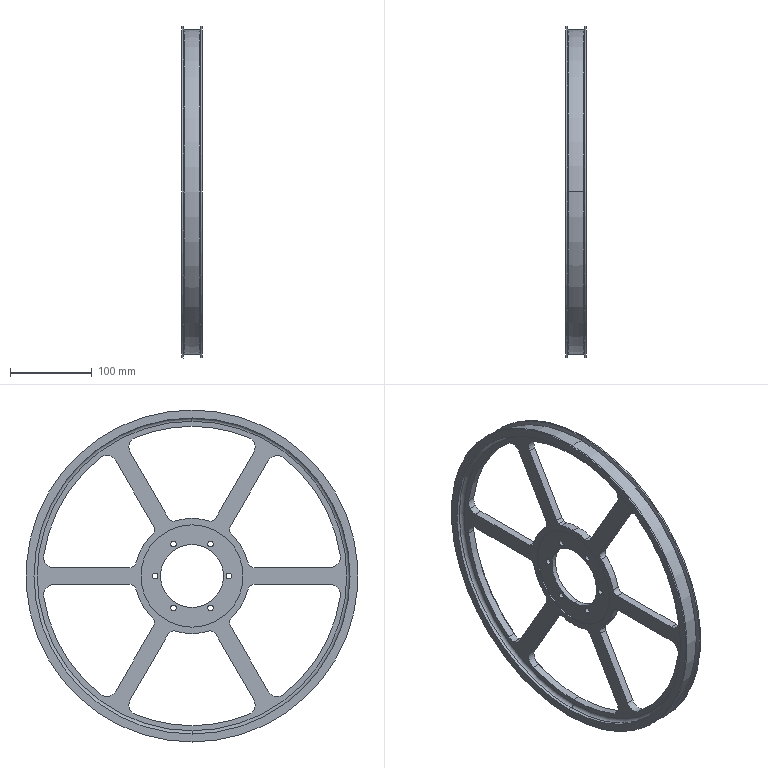Part | SolidWorks | features BaseBody 1 | 1 solid | 104 faces | box 25 x 405 x 405 mm | volume 510494 mm3 | cylinder 76 | plane 18 | torus 6 | cone 4 | commonest cylinder face diameters 15 x18 25 x16 7 x12 140.5 x8 365 x8 125 x4